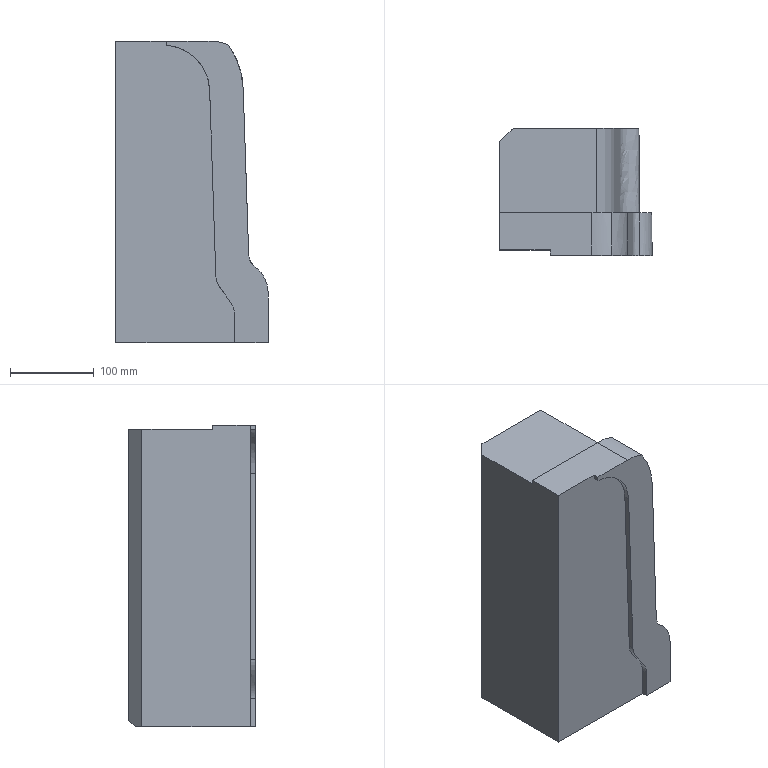Part | NX | features solid 2 | 1 solid | 22 faces | box 181.81 x 151.29 x 360.008 mm | volume 7698376 mm3 | spline 14 | plane 8